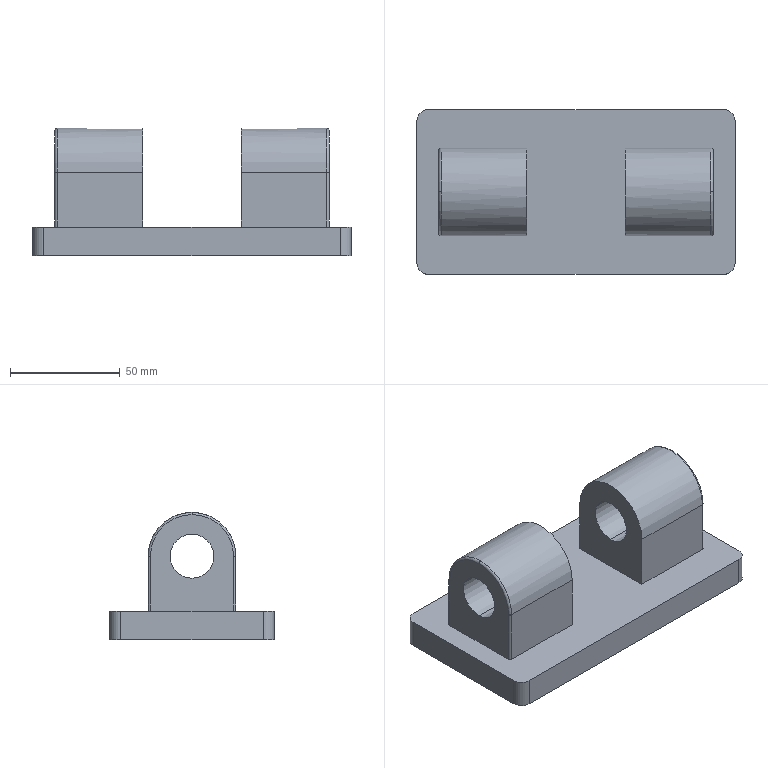Part | STEP file | Hinge lug widened | 1 solid | 32 faces | box 145 x 75 x 58 mm | volume 246181 mm3 | cylinder 14 | plane 14 | torus 4 | commonest cylinder face diameters 2 x4 10 x4 20 x4 40 x2
STEP:
#1=CARTESIAN_POINT('',(57.873,-48.431,650.5));
#2=VERTEX_POINT('',#1);
#3=CARTESIAN_POINT('',(57.873,-48.431,670.5));
#4=VERTEX_POINT('',#3);
#5=CARTESIAN_POINT('',(57.873,-48.431,660.5));
#6=DIRECTION('',(-1.,0.,0.));
#7=DIRECTION('',(0.,0.,1.));
#8=AXIS2_PLACEMENT_3D('',#5,#6,#7);
#9=CIRCLE('',#8,10.);
#10=EDGE_CURVE('',#2,#4,#9,.T.);
#11=ORIENTED_EDGE('',*,*,#10,.F.);
#12=CARTESIAN_POINT('',(17.873,-48.431,650.5));
#13=VERTEX_POINT('',#12);
#14=CARTESIAN_POINT('',(67.873,-48.431,650.5));
#15=DIRECTION('',(-1.,0.,0.));
#16=VECTOR('',#15,1000.);
#17=LINE('',#14,#16);
#18=EDGE_CURVE('',#2,#13,#17,.T.);
#19=ORIENTED_EDGE('',*,*,#18,.T.);
#20=CARTESIAN_POINT('',(17.873,-48.431,670.5));
#21=VERTEX_POINT('',#20);
#22=CARTESIAN_POINT('',(17.873,-48.431,660.5));
#23=DIRECTION('',(-1.,0.,0.));
#24=DIRECTION('',(0.,0.,-1.));
#25=AXIS2_PLACEMENT_3D('',#22,#23,#24);
#26=CIRCLE('',#25,10.);
#27=EDGE_CURVE('',#13,#21,#26,.T.);
#28=ORIENTED_EDGE('',*,*,#27,.T.);
#29=CARTESIAN_POINT('',(67.873,-48.431,670.5));
#30=DIRECTION('',(-1.,0.,0.));
#31=VECTOR('',#30,1000.);
#32=LINE('',#29,#31);
#33=EDGE_CURVE('',#4,#21,#32,.T.);
#34=ORIENTED_EDGE('',*,*,#33,.F.);
#35=EDGE_LOOP('',(#11,#19,#28,#34));
#36=FACE_OUTER_BOUND('',#35,.T.);
#37=CARTESIAN_POINT('',(67.873,-48.431,660.5));
#38=DIRECTION('',(-1.,0.,0.));
#39=DIRECTION('',(0.,0.,1.));
#40=AXIS2_PLACEMENT_3D('',#37,#38,#39);
#41=CYLINDRICAL_SURFACE('',#40,10.);
#42=ADVANCED_FACE('',(#36),#41,.F.);
#43=CARTESIAN_POINT('',(-27.127,-48.431,650.5));
#44=VERTEX_POINT('',#43);
#45=CARTESIAN_POINT('',(-27.127,-48.431,670.5));
#46=VERTEX_POINT('',#45);
#47=CARTESIAN_POINT('',(-27.127,-48.431,660.5));
#48=DIRECTION('',(-1.,0.,0.));
#49=DIRECTION('',(0.,0.,-1.));
#50=AXIS2_PLACEMENT_3D('',#47,#48,#49);
#51=CIRCLE('',#50,10.);
#52=EDGE_CURVE('',#44,#46,#51,.T.);
#53=ORIENTED_EDGE('',*,*,#52,.F.);
#54=CARTESIAN_POINT('',(-67.127,-48.431,650.5));
#55=VERTEX_POINT('',#54);
#56=CARTESIAN_POINT('',(7.873,-48.431,650.5));
#57=DIRECTION('',(-1.,0.,0.));
#58=VECTOR('',#57,1000.);
#59=LINE('',#56,#58);
#60=EDGE_CURVE('',#44,#55,#59,.T.);
#61=ORIENTED_EDGE('',*,*,#60,.T.);
#62=CARTESIAN_POINT('',(-67.127,-48.431,670.5));
#63=VERTEX_POINT('',#62);
#64=CARTESIAN_POINT('',(-67.127,-48.431,660.5));
#65=DIRECTION('',(-1.,0.,0.));
#66=DIRECTION('',(0.,0.,1.));
#67=AXIS2_PLACEMENT_3D('',#64,#65,#66);
#68=CIRCLE('',#67,10.);
#69=EDGE_CURVE('',#55,#63,#68,.T.);
#70=ORIENTED_EDGE('',*,*,#69,.T.);
#71=CARTESIAN_POINT('',(7.873,-48.431,670.5));
#72=DIRECTION('',(-1.,0.,0.));
#73=VECTOR('',#72,1000.);
#74=LINE('',#71,#73);
#75=EDGE_CURVE('',#46,#63,#74,.T.);
#76=ORIENTED_EDGE('',*,*,#75,.F.);
#77=EDGE_LOOP('',(#53,#61,#70,#76));
#78=FACE_OUTER_BOUND('',#77,.T.);
#79=CARTESIAN_POINT('',(7.873,-48.431,660.5));
#80=DIRECTION('',(-1.,0.,0.));
#81=DIRECTION('',(0.,0.,1.));
#82=AXIS2_PLACEMENT_3D('',#79,#80,#81);
#83=CYLINDRICAL_SURFACE('',#82,10.);
#84=ADVANCED_FACE('',(#78),#83,.F.);
#85=CARTESIAN_POINT('',(17.873,-28.431,635.5));
#86=VERTEX_POINT('',#85);
#87=CARTESIAN_POINT('',(17.873,-68.431,635.5));
#88=VERTEX_POINT('',#87);
#89=CARTESIAN_POINT('',(17.873,-58.431,635.5));
#90=DIRECTION('',(0.,-1.,0.));
#91=VECTOR('',#90,1000.);
#92=LINE('',#89,#91);
#93=EDGE_CURVE('',#86,#88,#92,.T.);
#94=ORIENTED_EDGE('',*,*,#93,.F.);
#95=CARTESIAN_POINT('',(56.873,-28.431,635.5));
#96=VERTEX_POINT('',#95);
#97=CARTESIAN_POINT('',(57.873,-28.431,635.5));
#98=DIRECTION('',(-1.,0.,0.));
#99=VECTOR('',#98,1000.);
#100=LINE('',#97,#99);
#101=EDGE_CURVE('',#96,#86,#100,.T.);
#102=ORIENTED_EDGE('',*,*,#101,.F.);
#103=CARTESIAN_POINT('',(57.873,-29.431,635.5));
#104=VERTEX_POINT('',#103);
#105=CARTESIAN_POINT('',(56.873,-29.431,635.5));
#106=DIRECTION('',(0.,0.,-1.));
#107=DIRECTION('',(1.,0.,0.));
#108=AXIS2_PLACEMENT_3D('',#105,#106,#107);
#109=CIRCLE('',#108,1.);
#110=EDGE_CURVE('',#96,#104,#109,.T.);
#111=ORIENTED_EDGE('',*,*,#110,.T.);
#112=CARTESIAN_POINT('',(57.873,-67.431,635.5));
#113=VERTEX_POINT('',#112);
#114=CARTESIAN_POINT('',(57.873,-28.431,635.5));
#115=DIRECTION('',(0.,1.,0.));
#116=VECTOR('',#115,1000.);
#117=LINE('',#114,#116);
#118=EDGE_CURVE('',#113,#104,#117,.T.);
#119=ORIENTED_EDGE('',*,*,#118,.F.);
#120=CARTESIAN_POINT('',(56.873,-68.431,635.5));
#121=VERTEX_POINT('',#120);
#122=CARTESIAN_POINT('',(56.873,-67.431,635.5));
#123=DIRECTION('',(0.,0.,-1.));
#124=DIRECTION('',(1.,0.,0.));
#125=AXIS2_PLACEMENT_3D('',#122,#123,#124);
#126=CIRCLE('',#125,1.);
#127=EDGE_CURVE('',#113,#121,#126,.T.);
#128=ORIENTED_EDGE('',*,*,#127,.T.);
#129=CARTESIAN_POINT('',(57.873,-68.431,635.5));
#130=DIRECTION('',(1.,0.,0.));
#131=VECTOR('',#130,1000.);
#132=LINE('',#129,#131);
#133=EDGE_CURVE('',#88,#121,#132,.T.);
#134=ORIENTED_EDGE('',*,*,#133,.F.);
#135=EDGE_LOOP('',(#94,#102,#111,#119,#128,#134));
#136=FACE_BOUND('',#135,.T.);
#137=CARTESIAN_POINT('',(62.873,-85.931,635.5));
#138=VERTEX_POINT('',#137);
#139=CARTESIAN_POINT('',(-72.127,-85.931,635.5));
#140=VERTEX_POINT('',#139);
#141=CARTESIAN_POINT('',(-77.127,-85.931,635.5));
#142=DIRECTION('',(-1.,0.,0.));
#143=VECTOR('',#142,1000.);
#144=LINE('',#141,#143);
#145=EDGE_CURVE('',#138,#140,#144,.T.);
#146=ORIENTED_EDGE('',*,*,#145,.F.);
#147=CARTESIAN_POINT('',(67.873,-80.931,635.5));
#148=VERTEX_POINT('',#147);
#149=CARTESIAN_POINT('',(62.873,-80.931,635.5));
#150=DIRECTION('',(0.,0.,1.));
#151=DIRECTION('',(1.,0.,0.));
#152=AXIS2_PLACEMENT_3D('',#149,#150,#151);
#153=CIRCLE('',#152,5.);
#154=EDGE_CURVE('',#138,#148,#153,.T.);
#155=ORIENTED_EDGE('',*,*,#154,.T.);
#156=CARTESIAN_POINT('',(67.873,-15.931,635.5));
#157=VERTEX_POINT('',#156);
#158=CARTESIAN_POINT('',(67.873,-10.931,635.5));
#159=DIRECTION('',(0.,-1.,0.));
#160=VECTOR('',#159,1000.);
#161=LINE('',#158,#160);
#162=EDGE_CURVE('',#157,#148,#161,.T.);
#163=ORIENTED_EDGE('',*,*,#162,.F.);
#164=CARTESIAN_POINT('',(62.873,-10.931,635.5));
#165=VERTEX_POINT('',#164);
#166=CARTESIAN_POINT('',(62.873,-15.931,635.5));
#167=DIRECTION('',(0.,0.,1.));
#168=DIRECTION('',(1.,0.,0.));
#169=AXIS2_PLACEMENT_3D('',#166,#167,#168);
#170=CIRCLE('',#169,5.);
#171=EDGE_CURVE('',#157,#165,#170,.T.);
#172=ORIENTED_EDGE('',*,*,#171,.T.);
#173=CARTESIAN_POINT('',(-72.127,-10.931,635.5));
#174=VERTEX_POINT('',#173);
#175=CARTESIAN_POINT('',(-77.127,-10.931,635.5));
#176=DIRECTION('',(1.,0.,0.));
#177=VECTOR('',#176,1000.);
#178=LINE('',#175,#177);
#179=EDGE_CURVE('',#174,#165,#178,.T.);
#180=ORIENTED_EDGE('',*,*,#179,.F.);
#181=CARTESIAN_POINT('',(-77.127,-15.931,635.5));
#182=VERTEX_POINT('',#181);
#183=CARTESIAN_POINT('',(-72.127,-15.931,635.5));
#184=DIRECTION('',(0.,0.,1.));
#185=DIRECTION('',(1.,0.,0.));
#186=AXIS2_PLACEMENT_3D('',#183,#184,#185);
#187=CIRCLE('',#186,5.);
#188=EDGE_CURVE('',#174,#182,#187,.T.);
#189=ORIENTED_EDGE('',*,*,#188,.T.);
#190=CARTESIAN_POINT('',(-77.127,-80.931,635.5));
#191=VERTEX_POINT('',#190);
#192=CARTESIAN_POINT('',(-77.127,-10.931,635.5));
#193=DIRECTION('',(0.,1.,0.));
#194=VECTOR('',#193,1000.);
#195=LINE('',#192,#194);
#196=EDGE_CURVE('',#191,#182,#195,.T.);
#197=ORIENTED_EDGE('',*,*,#196,.F.);
#198=CARTESIAN_POINT('',(-72.127,-80.931,635.5));
#199=DIRECTION('',(0.,0.,1.));
#200=DIRECTION('',(1.,0.,0.));
#201=AXIS2_PLACEMENT_3D('',#198,#199,#200);
#202=CIRCLE('',#201,5.);
#203=EDGE_CURVE('',#191,#140,#202,.T.);
#204=ORIENTED_EDGE('',*,*,#203,.T.);
#205=EDGE_LOOP('',(#146,#155,#163,#172,#180,#189,#197,#204));
#206=FACE_OUTER_BOUND('',#205,.T.);
#207=CARTESIAN_POINT('',(-27.127,-28.431,635.5));
#208=VERTEX_POINT('',#207);
#209=CARTESIAN_POINT('',(-66.127,-28.431,635.5));
#210=VERTEX_POINT('',#209);
#211=CARTESIAN_POINT('',(-67.127,-28.431,635.5));
#212=DIRECTION('',(-1.,0.,0.));
#213=VECTOR('',#212,1000.);
#214=LINE('',#211,#213);
#215=EDGE_CURVE('',#208,#210,#214,.T.);
#216=ORIENTED_EDGE('',*,*,#215,.F.);
#217=CARTESIAN_POINT('',(-27.127,-68.431,635.5));
#218=VERTEX_POINT('',#217);
#219=CARTESIAN_POINT('',(-27.127,-58.431,635.5));
#220=DIRECTION('',(0.,-1.,0.));
#221=VECTOR('',#220,1000.);
#222=LINE('',#219,#221);
#223=EDGE_CURVE('',#208,#218,#222,.T.);
#224=ORIENTED_EDGE('',*,*,#223,.T.);
#225=CARTESIAN_POINT('',(-66.127,-68.431,635.5));
#226=VERTEX_POINT('',#225);
#227=CARTESIAN_POINT('',(-67.127,-68.431,635.5));
#228=DIRECTION('',(1.,0.,0.));
#229=VECTOR('',#228,1000.);
#230=LINE('',#227,#229);
#231=EDGE_CURVE('',#226,#218,#230,.T.);
#232=ORIENTED_EDGE('',*,*,#231,.F.);
#233=CARTESIAN_POINT('',(-67.127,-67.431,635.5));
#234=VERTEX_POINT('',#233);
#235=CARTESIAN_POINT('',(-66.127,-67.431,635.5));
#236=DIRECTION('',(0.,0.,-1.));
#237=DIRECTION('',(1.,0.,0.));
#238=AXIS2_PLACEMENT_3D('',#235,#236,#237);
#239=CIRCLE('',#238,1.);
#240=EDGE_CURVE('',#226,#234,#239,.T.);
#241=ORIENTED_EDGE('',*,*,#240,.T.);
#242=CARTESIAN_POINT('',(-67.127,-29.431,635.5));
#243=VERTEX_POINT('',#242);
#244=CARTESIAN_POINT('',(-67.127,-28.431,635.5));
#245=DIRECTION('',(0.,-1.,0.));
#246=VECTOR('',#245,1000.);
#247=LINE('',#244,#246);
#248=EDGE_CURVE('',#243,#234,#247,.T.);
#249=ORIENTED_EDGE('',*,*,#248,.F.);
#250=CARTESIAN_POINT('',(-66.127,-29.431,635.5));
#251=DIRECTION('',(0.,0.,-1.));
#252=DIRECTION('',(1.,0.,0.));
#253=AXIS2_PLACEMENT_3D('',#250,#251,#252);
#254=CIRCLE('',#253,1.);
#255=EDGE_CURVE('',#243,#210,#254,.T.);
#256=ORIENTED_EDGE('',*,*,#255,.T.);
#257=EDGE_LOOP('',(#216,#224,#232,#241,#249,#256));
#258=FACE_BOUND('',#257,.T.);
#259=CARTESIAN_POINT('',(-34.627,-48.431,635.5));
#260=DIRECTION('',(0.,0.,1.));
#261=DIRECTION('',(0.,-1.,0.));
#262=AXIS2_PLACEMENT_3D('',#259,#260,#261);
#263=PLANE('',#262);
#264=ADVANCED_FACE('',(#136,#206,#258),#263,.T.);
#265=ORIENTED_EDGE('',*,*,#179,.T.);
#266=CARTESIAN_POINT('',(62.873,-10.931,622.5));
#267=VERTEX_POINT('',#266);
#268=CARTESIAN_POINT('',(62.873,-10.931,622.5));
#269=DIRECTION('',(0.,0.,-1.));
#270=VECTOR('',#269,1000.);
#271=LINE('',#268,#270);
#272=EDGE_CURVE('',#165,#267,#271,.T.);
#273=ORIENTED_EDGE('',*,*,#272,.T.);
#274=CARTESIAN_POINT('',(-72.127,-10.931,622.5));
#275=VERTEX_POINT('',#274);
#276=CARTESIAN_POINT('',(-77.127,-10.931,622.5));
#277=DIRECTION('',(1.,0.,0.));
#278=VECTOR('',#277,1000.);
#279=LINE('',#276,#278);
#280=EDGE_CURVE('',#275,#267,#279,.T.);
#281=ORIENTED_EDGE('',*,*,#280,.F.);
#282=CARTESIAN_POINT('',(-72.127,-10.931,622.5));
#283=DIRECTION('',(0.,0.,1.));
#284=VECTOR('',#283,1000.);
#285=LINE('',#282,#284);
#286=EDGE_CURVE('',#275,#174,#285,.T.);
#287=ORIENTED_EDGE('',*,*,#286,.T.);
#288=EDGE_LOOP('',(#265,#273,#281,#287));
#289=FACE_OUTER_BOUND('',#288,.T.);
#290=CARTESIAN_POINT('',(-77.127,-10.931,622.5));
#291=DIRECTION('',(0.,-1.,0.));
#292=DIRECTION('',(0.,0.,1.));
#293=AXIS2_PLACEMENT_3D('',#290,#291,#292);
#294=PLANE('',#293);
#295=ADVANCED_FACE('',(#289),#294,.F.);
#296=CARTESIAN_POINT('',(62.873,-85.931,622.5));
#297=VERTEX_POINT('',#296);
#298=CARTESIAN_POINT('',(-72.127,-85.931,622.5));
#299=VERTEX_POINT('',#298);
#300=CARTESIAN_POINT('',(-77.127,-85.931,622.5));
#301=DIRECTION('',(-1.,0.,0.));
#302=VECTOR('',#301,1000.);
#303=LINE('',#300,#302);
#304=EDGE_CURVE('',#297,#299,#303,.T.);
#305=ORIENTED_EDGE('',*,*,#304,.F.);
#306=CARTESIAN_POINT('',(62.873,-85.931,622.5));
#307=DIRECTION('',(0.,0.,1.));
#308=VECTOR('',#307,1000.);
#309=LINE('',#306,#308);
#310=EDGE_CURVE('',#297,#138,#309,.T.);
#311=ORIENTED_EDGE('',*,*,#310,.T.);
#312=ORIENTED_EDGE('',*,*,#145,.T.);
#313=CARTESIAN_POINT('',(-72.127,-85.931,622.5));
#314=DIRECTION('',(0.,0.,-1.));
#315=VECTOR('',#314,1000.);
#316=LINE('',#313,#315);
#317=EDGE_CURVE('',#140,#299,#316,.T.);
#318=ORIENTED_EDGE('',*,*,#317,.T.);
#319=EDGE_LOOP('',(#305,#311,#312,#318));
#320=FACE_OUTER_BOUND('',#319,.T.);
#321=CARTESIAN_POINT('',(-77.127,-85.931,622.5));
#322=DIRECTION('',(0.,1.,0.));
#323=DIRECTION('',(-1.,0.,0.));
#324=AXIS2_PLACEMENT_3D('',#321,#322,#323);
#325=PLANE('',#324);
#326=ADVANCED_FACE('',(#320),#325,.F.);
#327=ORIENTED_EDGE('',*,*,#280,.T.);
#328=CARTESIAN_POINT('',(67.873,-15.931,622.5));
#329=VERTEX_POINT('',#328);
#330=CARTESIAN_POINT('',(62.873,-15.931,622.5));
#331=DIRECTION('',(0.,0.,-1.));
#332=DIRECTION('',(1.,0.,0.));
#333=AXIS2_PLACEMENT_3D('',#330,#331,#332);
#334=CIRCLE('',#333,5.);
#335=EDGE_CURVE('',#267,#329,#334,.T.);
#336=ORIENTED_EDGE('',*,*,#335,.T.);
#337=CARTESIAN_POINT('',(67.873,-80.931,622.5));
#338=VERTEX_POINT('',#337);
#339=CARTESIAN_POINT('',(67.873,-10.931,622.5));
#340=DIRECTION('',(0.,-1.,0.));
#341=VECTOR('',#340,1000.);
#342=LINE('',#339,#341);
#343=EDGE_CURVE('',#329,#338,#342,.T.);
#344=ORIENTED_EDGE('',*,*,#343,.T.);
#345=CARTESIAN_POINT('',(62.873,-80.931,622.5));
#346=DIRECTION('',(0.,0.,-1.));
#347=DIRECTION('',(1.,0.,0.));
#348=AXIS2_PLACEMENT_3D('',#345,#346,#347);
#349=CIRCLE('',#348,5.);
#350=EDGE_CURVE('',#338,#297,#349,.T.);
#351=ORIENTED_EDGE('',*,*,#350,.T.);
#352=ORIENTED_EDGE('',*,*,#304,.T.);
#353=CARTESIAN_POINT('',(-77.127,-80.931,622.5));
#354=VERTEX_POINT('',#353);
#355=CARTESIAN_POINT('',(-72.127,-80.931,622.5));
#356=DIRECTION('',(0.,0.,-1.));
#357=DIRECTION('',(1.,0.,0.));
#358=AXIS2_PLACEMENT_3D('',#355,#356,#357);
#359=CIRCLE('',#358,5.);
#360=EDGE_CURVE('',#299,#354,#359,.T.);
#361=ORIENTED_EDGE('',*,*,#360,.T.);
#362=CARTESIAN_POINT('',(-77.127,-15.931,622.5));
#363=VERTEX_POINT('',#362);
#364=CARTESIAN_POINT('',(-77.127,-10.931,622.5));
#365=DIRECTION('',(0.,1.,0.));
#366=VECTOR('',#365,1000.);
#367=LINE('',#364,#366);
#368=EDGE_CURVE('',#354,#363,#367,.T.);
#369=ORIENTED_EDGE('',*,*,#368,.T.);
#370=CARTESIAN_POINT('',(-72.127,-15.931,622.5));
#371=DIRECTION('',(0.,0.,-1.));
#372=DIRECTION('',(1.,0.,0.));
#373=AXIS2_PLACEMENT_3D('',#370,#371,#372);
#374=CIRCLE('',#373,5.);
#375=EDGE_CURVE('',#363,#275,#374,.T.);
#376=ORIENTED_EDGE('',*,*,#375,.T.);
#377=EDGE_LOOP('',(#327,#336,#344,#351,#352,#361,#369,#376));
#378=FACE_OUTER_BOUND('',#377,.T.);
#379=CARTESIAN_POINT('',(-34.627,-48.431,622.5));
#380=DIRECTION('',(0.,0.,1.));
#381=DIRECTION('',(0.,-1.,0.));
#382=AXIS2_PLACEMENT_3D('',#379,#380,#381);
#383=PLANE('',#382);
#384=ADVANCED_FACE('',(#378),#383,.F.);
#385=ORIENTED_EDGE('',*,*,#60,.F.);
#386=CARTESIAN_POINT('',(-27.127,-48.431,660.5));
#387=DIRECTION('',(-1.,0.,0.));
#388=DIRECTION('',(0.,0.,-1.));
#389=AXIS2_PLACEMENT_3D('',#386,#387,#388);
#390=CIRCLE('',#389,10.);
#391=EDGE_CURVE('',#46,#44,#390,.T.);
#392=ORIENTED_EDGE('',*,*,#391,.F.);
#393=ORIENTED_EDGE('',*,*,#75,.T.);
#394=CARTESIAN_POINT('',(-67.127,-48.431,660.5));
#395=DIRECTION('',(-1.,0.,0.));
#396=DIRECTION('',(0.,0.,1.));
#397=AXIS2_PLACEMENT_3D('',#394,#395,#396);
#398=CIRCLE('',#397,10.);
#399=EDGE_CURVE('',#63,#55,#398,.T.);
#400=ORIENTED_EDGE('',*,*,#399,.T.);
#401=EDGE_LOOP('',(#385,#392,#393,#400));
#402=FACE_OUTER_BOUND('',#401,.T.);
#403=CARTESIAN_POINT('',(7.873,-48.431,660.5));
#404=DIRECTION('',(-1.,0.,0.));
#405=DIRECTION('',(0.,0.,1.));
#406=AXIS2_PLACEMENT_3D('',#403,#404,#405);
#407=CYLINDRICAL_SURFACE('',#406,10.);
#408=ADVANCED_FACE('',(#402),#407,.F.);
#409=ORIENTED_EDGE('',*,*,#196,.T.);
#410=CARTESIAN_POINT('',(-77.127,-15.931,622.5));
#411=DIRECTION('',(0.,0.,-1.));
#412=VECTOR('',#411,1000.);
#413=LINE('',#410,#412);
#414=EDGE_CURVE('',#182,#363,#413,.T.);
#415=ORIENTED_EDGE('',*,*,#414,.T.);
#416=ORIENTED_EDGE('',*,*,#368,.F.);
#417=CARTESIAN_POINT('',(-77.127,-80.931,622.5));
#418=DIRECTION('',(0.,0.,1.));
#419=VECTOR('',#418,1000.);
#420=LINE('',#417,#419);
#421=EDGE_CURVE('',#354,#191,#420,.T.);
#422=ORIENTED_EDGE('',*,*,#421,.T.);
#423=EDGE_LOOP('',(#409,#415,#416,#422));
#424=FACE_OUTER_BOUND('',#423,.T.);
#425=CARTESIAN_POINT('',(-77.127,-10.931,622.5));
#426=DIRECTION('',(1.,0.,0.));
#427=DIRECTION('',(0.,1.,0.));
#428=AXIS2_PLACEMENT_3D('',#425,#426,#427);
#429=PLANE('',#428);
#430=ADVANCED_FACE('',(#424),#429,.F.);
#431=ORIENTED_EDGE('',*,*,#248,.T.);
#432=CARTESIAN_POINT('',(-67.127,-67.431,660.5));
#433=VERTEX_POINT('',#432);
#434=CARTESIAN_POINT('',(-67.127,-67.431,680.5));
#435=DIRECTION('',(0.,0.,1.));
#436=VECTOR('',#435,1000.);
#437=LINE('',#434,#436);
#438=EDGE_CURVE('',#234,#433,#437,.T.);
#439=ORIENTED_EDGE('',*,*,#438,.T.);
#440=CARTESIAN_POINT('',(-67.127,-48.431,679.5));
#441=VERTEX_POINT('',#440);
#442=CARTESIAN_POINT('',(-67.127,-48.431,660.5));
#443=DIRECTION('',(-1.,0.,0.));
#444=DIRECTION('',(0.,0.,-1.));
#445=AXIS2_PLACEMENT_3D('',#442,#443,#444);
#446=CIRCLE('',#445,19.);
#447=EDGE_CURVE('',#433,#441,#446,.T.);
#448=ORIENTED_EDGE('',*,*,#447,.T.);
#449=CARTESIAN_POINT('',(-67.127,-29.431,660.5));
#450=VERTEX_POINT('',#449);
#451=CARTESIAN_POINT('',(-67.127,-48.431,660.5));
#452=DIRECTION('',(-1.,0.,0.));
#453=DIRECTION('',(0.,0.,-1.));
#454=AXIS2_PLACEMENT_3D('',#451,#452,#453);
#455=CIRCLE('',#454,19.);
#456=EDGE_CURVE('',#441,#450,#455,.T.);
#457=ORIENTED_EDGE('',*,*,#456,.T.);
#458=CARTESIAN_POINT('',(-67.127,-29.431,680.5));
#459=DIRECTION('',(0.,0.,-1.));
#460=VECTOR('',#459,1000.);
#461=LINE('',#458,#460);
#462=EDGE_CURVE('',#450,#243,#461,.T.);
#463=ORIENTED_EDGE('',*,*,#462,.T.);
#464=EDGE_LOOP('',(#431,#439,#448,#457,#463));
#465=FACE_OUTER_BOUND('',#464,.T.);
#466=ORIENTED_EDGE('',*,*,#399,.F.);
#467=ORIENTED_EDGE('',*,*,#69,.F.);
#468=EDGE_LOOP('',(#466,#467));
#469=FACE_BOUND('',#468,.T.);
#470=CARTESIAN_POINT('',(-67.127,-28.431,680.5));
#471=DIRECTION('',(1.,0.,0.));
#472=DIRECTION('',(0.,0.,-1.));
#473=AXIS2_PLACEMENT_3D('',#470,#471,#472);
#474=PLANE('',#473);
#475=ADVANCED_FACE('',(#465,#469),#474,.F.);
#476=ORIENTED_EDGE('',*,*,#231,.T.);
#477=CARTESIAN_POINT('',(-27.127,-68.431,660.5));
#478=VERTEX_POINT('',#477);
#479=CARTESIAN_POINT('',(-27.127,-68.431,635.5));
#480=DIRECTION('',(0.,0.,1.));
#481=VECTOR('',#480,1000.);
#482=LINE('',#479,#481);
#483=EDGE_CURVE('',#218,#478,#482,.T.);
#484=ORIENTED_EDGE('',*,*,#483,.T.);
#485=CARTESIAN_POINT('',(-66.127,-68.431,660.5));
#486=VERTEX_POINT('',#485);
#487=CARTESIAN_POINT('',(-67.127,-68.431,660.5));
#488=DIRECTION('',(-1.,0.,0.));
#489=VECTOR('',#488,1000.);
#490=LINE('',#487,#489);
#491=EDGE_CURVE('',#478,#486,#490,.T.);
#492=ORIENTED_EDGE('',*,*,#491,.T.);
#493=CARTESIAN_POINT('',(-66.127,-68.431,680.5));
#494=DIRECTION('',(0.,0.,-1.));
#495=VECTOR('',#494,1000.);
#496=LINE('',#493,#495);
#497=EDGE_CURVE('',#486,#226,#496,.T.);
#498=ORIENTED_EDGE('',*,*,#497,.T.);
#499=EDGE_LOOP('',(#476,#484,#492,#498));
#500=FACE_OUTER_BOUND('',#499,.T.);
#501=CARTESIAN_POINT('',(-67.127,-68.431,680.5));
#502=DIRECTION('',(0.,1.,0.));
#503=DIRECTION('',(-1.,0.,0.));
#504=AXIS2_PLACEMENT_3D('',#501,#502,#503);
#505=PLANE('',#504);
#506=ADVANCED_FACE('',(#500),#505,.F.);
#507=CARTESIAN_POINT('',(-66.127,-28.431,660.5));
#508=VERTEX_POINT('',#507);
#509=CARTESIAN_POINT('',(-27.127,-28.431,660.5));
#510=VERTEX_POINT('',#509);
#511=CARTESIAN_POINT('',(-47.127,-28.431,660.5));
#512=DIRECTION('',(1.,0.,0.));
#513=VECTOR('',#512,1000.);
#514=LINE('',#511,#513);
#515=EDGE_CURVE('',#508,#510,#514,.T.);
#516=ORIENTED_EDGE('',*,*,#515,.T.);
#517=CARTESIAN_POINT('',(-27.127,-28.431,660.5));
#518=DIRECTION('',(0.,0.,-1.));
#519=VECTOR('',#518,1000.);
#520=LINE('',#517,#519);
#521=EDGE_CURVE('',#510,#208,#520,.T.);
#522=ORIENTED_EDGE('',*,*,#521,.T.);
#523=ORIENTED_EDGE('',*,*,#215,.T.);
#524=CARTESIAN_POINT('',(-66.127,-28.431,680.5));
#525=DIRECTION('',(0.,0.,1.));
#526=VECTOR('',#525,1000.);
#527=LINE('',#524,#526);
#528=EDGE_CURVE('',#210,#508,#527,.T.);
#529=ORIENTED_EDGE('',*,*,#528,.T.);
#530=EDGE_LOOP('',(#516,#522,#523,#529));
#531=FACE_OUTER_BOUND('',#530,.T.);
#532=CARTESIAN_POINT('',(-67.127,-28.431,680.5));
#533=DIRECTION('',(0.,-1.,0.));
#534=DIRECTION('',(0.,0.,1.));
#535=AXIS2_PLACEMENT_3D('',#532,#533,#534);
#536=PLANE('',#535);
#537=ADVANCED_FACE('',(#531),#536,.F.);
#538=CARTESIAN_POINT('',(-66.127,-48.431,680.5));
#539=VERTEX_POINT('',#538);
#540=CARTESIAN_POINT('',(-66.127,-48.431,660.5));
#541=DIRECTION('',(1.,0.,0.));
#542=DIRECTION('',(0.,0.,-1.));
#543=AXIS2_PLACEMENT_3D('',#540,#541,#542);
#544=CIRCLE('',#543,20.);
#545=EDGE_CURVE('',#508,#539,#544,.T.);
#546=ORIENTED_EDGE('',*,*,#545,.T.);
#547=CARTESIAN_POINT('',(-66.127,-48.431,660.5));
#548=DIRECTION('',(1.,0.,0.));
#549=DIRECTION('',(0.,0.,-1.));
#550=AXIS2_PLACEMENT_3D('',#547,#548,#549);
#551=CIRCLE('',#550,20.);
#552=EDGE_CURVE('',#539,#486,#551,.T.);
#553=ORIENTED_EDGE('',*,*,#552,.T.);
#554=ORIENTED_EDGE('',*,*,#491,.F.);
#555=CARTESIAN_POINT('',(-27.127,-48.431,660.5));
#556=DIRECTION('',(-1.,0.,0.));
#557=DIRECTION('',(0.,0.,-1.));
#558=AXIS2_PLACEMENT_3D('',#555,#556,#557);
#559=CIRCLE('',#558,20.);
#560=EDGE_CURVE('',#478,#510,#559,.T.);
#561=ORIENTED_EDGE('',*,*,#560,.T.);
#562=ORIENTED_EDGE('',*,*,#515,.F.);
#563=EDGE_LOOP('',(#546,#553,#554,#561,#562));
#564=FACE_OUTER_BOUND('',#563,.T.);
#565=CARTESIAN_POINT('',(-34.627,-48.431,660.5));
#566=DIRECTION('',(1.,0.,0.));
#567=DIRECTION('',(0.,0.,-1.));
#568=AXIS2_PLACEMENT_3D('',#565,#566,#567);
#569=CYLINDRICAL_SURFACE('',#568,20.);
#570=ADVANCED_FACE('',(#564),#569,.T.);
#571=ORIENTED_EDGE('',*,*,#255,.F.);
#572=ORIENTED_EDGE('',*,*,#462,.F.);
#573=CARTESIAN_POINT('',(-66.127,-29.431,660.5));
#574=DIRECTION('',(0.,0.,1.));
#575=DIRECTION('',(1.,0.,0.));
#576=AXIS2_PLACEMENT_3D('',#573,#574,#575);
#577=CIRCLE('',#576,1.);
#578=EDGE_CURVE('',#508,#450,#577,.T.);
#579=ORIENTED_EDGE('',*,*,#578,.F.);
#580=ORIENTED_EDGE('',*,*,#528,.F.);
#581=EDGE_LOOP('',(#571,#572,#579,#580));
#582=FACE_OUTER_BOUND('',#581,.T.);
#583=CARTESIAN_POINT('',(-66.127,-29.431,680.5));
#584=DIRECTION('',(0.,0.,-1.));
#585=DIRECTION('',(-1.,0.,0.));
#586=AXIS2_PLACEMENT_3D('',#583,#584,#585);
#587=CYLINDRICAL_SURFACE('',#586,1.);
#588=ADVANCED_FACE('',(#582),#587,.T.);
#589=ORIENTED_EDGE('',*,*,#578,.T.);
#590=ORIENTED_EDGE('',*,*,#456,.F.);
#591=CARTESIAN_POINT('',(-66.127,-48.431,679.5));
#592=DIRECTION('',(0.,-1.,0.));
#593=DIRECTION('',(-1.,0.,0.));
#594=AXIS2_PLACEMENT_3D('',#591,#592,#593);
#595=CIRCLE('',#594,1.);
#596=EDGE_CURVE('',#539,#441,#595,.T.);
#597=ORIENTED_EDGE('',*,*,#596,.F.);
#598=ORIENTED_EDGE('',*,*,#545,.F.);
#599=EDGE_LOOP('',(#589,#590,#597,#598));
#600=FACE_OUTER_BOUND('',#599,.T.);
#601=CARTESIAN_POINT('',(-66.127,-48.431,660.5));
#602=DIRECTION('',(1.,0.,0.));
#603=DIRECTION('',(0.,0.,-1.));
#604=AXIS2_PLACEMENT_3D('',#601,#602,#603);
#605=TOROIDAL_SURFACE('',#604,19.,1.);
#606=ADVANCED_FACE('',(#600),#605,.T.);
#607=ORIENTED_EDGE('',*,*,#596,.T.);
#608=ORIENTED_EDGE('',*,*,#447,.F.);
#609=CARTESIAN_POINT('',(-66.127,-67.431,660.5));
#610=DIRECTION('',(0.,0.,-1.));
#611=DIRECTION('',(-1.,0.,0.));
#612=AXIS2_PLACEMENT_3D('',#609,#610,#611);
#613=CIRCLE('',#612,1.);
#614=EDGE_CURVE('',#486,#433,#613,.T.);
#615=ORIENTED_EDGE('',*,*,#614,.F.);
#616=ORIENTED_EDGE('',*,*,#552,.F.);
#617=EDGE_LOOP('',(#607,#608,#615,#616));
#618=FACE_OUTER_BOUND('',#617,.T.);
#619=CARTESIAN_POINT('',(-66.127,-48.431,660.5));
#620=DIRECTION('',(1.,0.,0.));
#621=DIRECTION('',(0.,0.,-1.));
#622=AXIS2_PLACEMENT_3D('',#619,#620,#621);
#623=TOROIDAL_SURFACE('',#622,19.,1.);
#624=ADVANCED_FACE('',(#618),#623,.T.);
#625=ORIENTED_EDGE('',*,*,#614,.T.);
#626=ORIENTED_EDGE('',*,*,#438,.F.);
#627=ORIENTED_EDGE('',*,*,#240,.F.);
#628=ORIENTED_EDGE('',*,*,#497,.F.);
#629=EDGE_LOOP('',(#625,#626,#627,#628));
#630=FACE_OUTER_BOUND('',#629,.T.);
#631=CARTESIAN_POINT('',(-66.127,-67.431,680.5));
#632=DIRECTION('',(0.,0.,-1.));
#633=DIRECTION('',(-1.,0.,0.));
#634=AXIS2_PLACEMENT_3D('',#631,#632,#633);
#635=CYLINDRICAL_SURFACE('',#634,1.);
#636=ADVANCED_FACE('',(#630),#635,.T.);
#637=ORIENTED_EDGE('',*,*,#375,.F.);
#638=ORIENTED_EDGE('',*,*,#414,.F.);
#639=ORIENTED_EDGE('',*,*,#188,.F.);
#640=ORIENTED_EDGE('',*,*,#286,.F.);
#641=EDGE_LOOP('',(#637,#638,#639,#640));
#642=FACE_OUTER_BOUND('',#641,.T.);
#643=CARTESIAN_POINT('',(-72.127,-15.931,622.5));
#644=DIRECTION('',(0.,0.,1.));
#645=DIRECTION('',(1.,0.,0.));
#646=AXIS2_PLACEMENT_3D('',#643,#644,#645);
#647=CYLINDRICAL_SURFACE('',#646,5.);
#648=ADVANCED_FACE('',(#642),#647,.T.);
#649=ORIENTED_EDGE('',*,*,#360,.F.);
#650=ORIENTED_EDGE('',*,*,#317,.F.);
#651=ORIENTED_EDGE('',*,*,#203,.F.);
#652=ORIENTED_EDGE('',*,*,#421,.F.);
#653=EDGE_LOOP('',(#649,#650,#651,#652));
#654=FACE_OUTER_BOUND('',#653,.T.);
#655=CARTESIAN_POINT('',(-72.127,-80.931,622.5));
#656=DIRECTION('',(0.,0.,1.));
#657=DIRECTION('',(1.,0.,0.));
#658=AXIS2_PLACEMENT_3D('',#655,#656,#657);
#659=CYLINDRICAL_SURFACE('',#658,5.);
#660=ADVANCED_FACE('',(#654),#659,.T.);
#661=CARTESIAN_POINT('',(56.873,-68.431,660.5));
#662=VERTEX_POINT('',#661);
#663=CARTESIAN_POINT('',(17.873,-68.431,660.5));
#664=VERTEX_POINT('',#663);
#665=CARTESIAN_POINT('',(57.873,-68.431,660.5));
#666=DIRECTION('',(-1.,0.,0.));
#667=VECTOR('',#666,1000.);
#668=LINE('',#665,#667);
#669=EDGE_CURVE('',#662,#664,#668,.T.);
#670=ORIENTED_EDGE('',*,*,#669,.F.);
#671=CARTESIAN_POINT('',(56.873,-48.431,680.5));
#672=VERTEX_POINT('',#671);
#673=CARTESIAN_POINT('',(56.873,-48.431,660.5));
#674=DIRECTION('',(-1.,0.,0.));
#675=DIRECTION('',(0.,0.,1.));
#676=AXIS2_PLACEMENT_3D('',#673,#674,#675);
#677=CIRCLE('',#676,20.);
#678=EDGE_CURVE('',#662,#672,#677,.T.);
#679=ORIENTED_EDGE('',*,*,#678,.T.);
#680=CARTESIAN_POINT('',(56.873,-28.431,660.5));
#681=VERTEX_POINT('',#680);
#682=CARTESIAN_POINT('',(56.873,-48.431,660.5));
#683=DIRECTION('',(-1.,0.,0.));
#684=DIRECTION('',(0.,0.,1.));
#685=AXIS2_PLACEMENT_3D('',#682,#683,#684);
#686=CIRCLE('',#685,20.);
#687=EDGE_CURVE('',#672,#681,#686,.T.);
#688=ORIENTED_EDGE('',*,*,#687,.T.);
#689=CARTESIAN_POINT('',(17.873,-28.431,660.5));
#690=VERTEX_POINT('',#689);
#691=CARTESIAN_POINT('',(57.873,-28.431,660.5));
#692=DIRECTION('',(1.,0.,0.));
#693=VECTOR('',#692,1000.);
#694=LINE('',#691,#693);
#695=EDGE_CURVE('',#690,#681,#694,.T.);
#696=ORIENTED_EDGE('',*,*,#695,.F.);
#697=CARTESIAN_POINT('',(17.873,-48.431,660.5));
#698=DIRECTION('',(-1.,0.,0.));
#699=DIRECTION('',(0.,0.,-1.));
#700=AXIS2_PLACEMENT_3D('',#697,#698,#699);
#701=CIRCLE('',#700,20.);
#702=EDGE_CURVE('',#664,#690,#701,.T.);
#703=ORIENTED_EDGE('',*,*,#702,.F.);
#704=EDGE_LOOP('',(#670,#679,#688,#696,#703));
#705=FACE_OUTER_BOUND('',#704,.T.);
#706=CARTESIAN_POINT('',(25.373,-48.431,660.5));
#707=DIRECTION('',(1.,0.,0.));
#708=DIRECTION('',(0.,-1.,0.));
#709=AXIS2_PLACEMENT_3D('',#706,#707,#708);
#710=CYLINDRICAL_SURFACE('',#709,20.);
#711=ADVANCED_FACE('',(#705),#710,.T.);
#712=ORIENTED_EDGE('',*,*,#18,.F.);
#713=CARTESIAN_POINT('',(57.873,-48.431,660.5));
#714=DIRECTION('',(-1.,0.,0.));
#715=DIRECTION('',(0.,0.,1.));
#716=AXIS2_PLACEMENT_3D('',#713,#714,#715);
#717=CIRCLE('',#716,10.);
#718=EDGE_CURVE('',#4,#2,#717,.T.);
#719=ORIENTED_EDGE('',*,*,#718,.F.);
#720=ORIENTED_EDGE('',*,*,#33,.T.);
#721=CARTESIAN_POINT('',(17.873,-48.431,660.5));
#722=DIRECTION('',(-1.,0.,0.));
#723=DIRECTION('',(0.,0.,-1.));
#724=AXIS2_PLACEMENT_3D('',#721,#722,#723);
#725=CIRCLE('',#724,10.);
#726=EDGE_CURVE('',#21,#13,#725,.T.);
#727=ORIENTED_EDGE('',*,*,#726,.T.);
#728=EDGE_LOOP('',(#712,#719,#720,#727));
#729=FACE_OUTER_BOUND('',#728,.T.);
#730=CARTESIAN_POINT('',(67.873,-48.431,660.5));
#731=DIRECTION('',(-1.,0.,0.));
#732=DIRECTION('',(0.,0.,1.));
#733=AXIS2_PLACEMENT_3D('',#730,#731,#732);
#734=CYLINDRICAL_SURFACE('',#733,10.);
#735=ADVANCED_FACE('',(#729),#734,.F.);
#736=CARTESIAN_POINT('',(57.873,-67.431,660.5));
#737=VERTEX_POINT('',#736);
#738=CARTESIAN_POINT('',(56.873,-67.431,660.5));
#739=DIRECTION('',(0.,0.,1.));
#740=DIRECTION('',(1.,0.,0.));
#741=AXIS2_PLACEMENT_3D('',#738,#739,#740);
#742=CIRCLE('',#741,1.);
#743=EDGE_CURVE('',#662,#737,#742,.T.);
#744=ORIENTED_EDGE('',*,*,#743,.T.);
#745=CARTESIAN_POINT('',(57.873,-48.431,679.5));
#746=VERTEX_POINT('',#745);
#747=CARTESIAN_POINT('',(57.873,-48.431,660.5));
#748=DIRECTION('',(1.,0.,0.));
#749=DIRECTION('',(0.,0.,1.));
#750=AXIS2_PLACEMENT_3D('',#747,#748,#749);
#751=CIRCLE('',#750,19.);
#752=EDGE_CURVE('',#746,#737,#751,.T.);
#753=ORIENTED_EDGE('',*,*,#752,.F.);
#754=CARTESIAN_POINT('',(56.873,-48.431,679.5));
#755=DIRECTION('',(0.,1.,0.));
#756=DIRECTION('',(0.,0.,-1.));
#757=AXIS2_PLACEMENT_3D('',#754,#755,#756);
#758=CIRCLE('',#757,1.);
#759=EDGE_CURVE('',#672,#746,#758,.T.);
#760=ORIENTED_EDGE('',*,*,#759,.F.);
#761=ORIENTED_EDGE('',*,*,#678,.F.);
#762=EDGE_LOOP('',(#744,#753,#760,#761));
#763=FACE_OUTER_BOUND('',#762,.T.);
#764=CARTESIAN_POINT('',(56.873,-48.431,660.5));
#765=DIRECTION('',(-1.,0.,0.));
#766=DIRECTION('',(0.,0.,1.));
#767=AXIS2_PLACEMENT_3D('',#764,#765,#766);
#768=TOROIDAL_SURFACE('',#767,19.,1.);
#769=ADVANCED_FACE('',(#763),#768,.T.);
#770=ORIENTED_EDGE('',*,*,#759,.T.);
#771=CARTESIAN_POINT('',(57.873,-29.431,660.5));
#772=VERTEX_POINT('',#771);
#773=CARTESIAN_POINT('',(57.873,-48.431,660.5));
#774=DIRECTION('',(1.,0.,0.));
#775=DIRECTION('',(0.,0.,1.));
#776=AXIS2_PLACEMENT_3D('',#773,#774,#775);
#777=CIRCLE('',#776,19.);
#778=EDGE_CURVE('',#772,#746,#777,.T.);
#779=ORIENTED_EDGE('',*,*,#778,.F.);
#780=CARTESIAN_POINT('',(56.873,-29.431,660.5));
#781=DIRECTION('',(0.,0.,-1.));
#782=DIRECTION('',(-1.,0.,0.));
#783=AXIS2_PLACEMENT_3D('',#780,#781,#782);
#784=CIRCLE('',#783,1.);
#785=EDGE_CURVE('',#681,#772,#784,.T.);
#786=ORIENTED_EDGE('',*,*,#785,.F.);
#787=ORIENTED_EDGE('',*,*,#687,.F.);
#788=EDGE_LOOP('',(#770,#779,#786,#787));
#789=FACE_OUTER_BOUND('',#788,.T.);
#790=CARTESIAN_POINT('',(56.873,-48.431,660.5));
#791=DIRECTION('',(-1.,0.,0.));
#792=DIRECTION('',(0.,0.,1.));
#793=AXIS2_PLACEMENT_3D('',#790,#791,#792);
#794=TOROIDAL_SURFACE('',#793,19.,1.);
#795=ADVANCED_FACE('',(#789),#794,.T.);
#796=ORIENTED_EDGE('',*,*,#133,.T.);
#797=CARTESIAN_POINT('',(56.873,-68.431,680.5));
#798=DIRECTION('',(0.,0.,1.));
#799=VECTOR('',#798,1000.);
#800=LINE('',#797,#799);
#801=EDGE_CURVE('',#121,#662,#800,.T.);
#802=ORIENTED_EDGE('',*,*,#801,.T.);
#803=ORIENTED_EDGE('',*,*,#669,.T.);
#804=CARTESIAN_POINT('',(17.873,-68.431,635.5));
#805=DIRECTION('',(0.,0.,1.));
#806=VECTOR('',#805,1000.);
#807=LINE('',#804,#806);
#808=EDGE_CURVE('',#88,#664,#807,.T.);
#809=ORIENTED_EDGE('',*,*,#808,.F.);
#810=EDGE_LOOP('',(#796,#802,#803,#809));
#811=FACE_OUTER_BOUND('',#810,.T.);
#812=CARTESIAN_POINT('',(57.873,-68.431,680.5));
#813=DIRECTION('',(0.,1.,0.));
#814=DIRECTION('',(-1.,0.,0.));
#815=AXIS2_PLACEMENT_3D('',#812,#813,#814);
#816=PLANE('',#815);
#817=ADVANCED_FACE('',(#811),#816,.F.);
#818=ORIENTED_EDGE('',*,*,#127,.F.);
#819=CARTESIAN_POINT('',(57.873,-67.431,680.5));
#820=DIRECTION('',(0.,0.,-1.));
#821=VECTOR('',#820,1000.);
#822=LINE('',#819,#821);
#823=EDGE_CURVE('',#737,#113,#822,.T.);
#824=ORIENTED_EDGE('',*,*,#823,.F.);
#825=ORIENTED_EDGE('',*,*,#743,.F.);
#826=ORIENTED_EDGE('',*,*,#801,.F.);
#827=EDGE_LOOP('',(#818,#824,#825,#826));
#828=FACE_OUTER_BOUND('',#827,.T.);
#829=CARTESIAN_POINT('',(56.873,-67.431,680.5));
#830=DIRECTION('',(0.,0.,-1.));
#831=DIRECTION('',(-1.,0.,0.));
#832=AXIS2_PLACEMENT_3D('',#829,#830,#831);
#833=CYLINDRICAL_SURFACE('',#832,1.);
#834=ADVANCED_FACE('',(#828),#833,.T.);
#835=ORIENTED_EDGE('',*,*,#118,.T.);
#836=CARTESIAN_POINT('',(57.873,-29.431,680.5));
#837=DIRECTION('',(0.,0.,1.));
#838=VECTOR('',#837,1000.);
#839=LINE('',#836,#838);
#840=EDGE_CURVE('',#104,#772,#839,.T.);
#841=ORIENTED_EDGE('',*,*,#840,.T.);
#842=ORIENTED_EDGE('',*,*,#778,.T.);
#843=ORIENTED_EDGE('',*,*,#752,.T.);
#844=ORIENTED_EDGE('',*,*,#823,.T.);
#845=EDGE_LOOP('',(#835,#841,#842,#843,#844));
#846=FACE_OUTER_BOUND('',#845,.T.);
#847=ORIENTED_EDGE('',*,*,#718,.T.);
#848=ORIENTED_EDGE('',*,*,#10,.T.);
#849=EDGE_LOOP('',(#847,#848));
#850=FACE_BOUND('',#849,.T.);
#851=CARTESIAN_POINT('',(57.873,-28.431,680.5));
#852=DIRECTION('',(-1.,0.,0.));
#853=DIRECTION('',(0.,1.,0.));
#854=AXIS2_PLACEMENT_3D('',#851,#852,#853);
#855=PLANE('',#854);
#856=ADVANCED_FACE('',(#846,#850),#855,.F.);
#857=ORIENTED_EDGE('',*,*,#785,.T.);
#858=ORIENTED_EDGE('',*,*,#840,.F.);
#859=ORIENTED_EDGE('',*,*,#110,.F.);
#860=CARTESIAN_POINT('',(56.873,-28.431,680.5));
#861=DIRECTION('',(0.,0.,-1.));
#862=VECTOR('',#861,1000.);
#863=LINE('',#860,#862);
#864=EDGE_CURVE('',#681,#96,#863,.T.);
#865=ORIENTED_EDGE('',*,*,#864,.F.);
#866=EDGE_LOOP('',(#857,#858,#859,#865));
#867=FACE_OUTER_BOUND('',#866,.T.);
#868=CARTESIAN_POINT('',(56.873,-29.431,680.5));
#869=DIRECTION('',(0.,0.,-1.));
#870=DIRECTION('',(-1.,0.,0.));
#871=AXIS2_PLACEMENT_3D('',#868,#869,#870);
#872=CYLINDRICAL_SURFACE('',#871,1.);
#873=ADVANCED_FACE('',(#867),#872,.T.);
#874=ORIENTED_EDGE('',*,*,#695,.T.);
#875=ORIENTED_EDGE('',*,*,#864,.T.);
#876=ORIENTED_EDGE('',*,*,#101,.T.);
#877=CARTESIAN_POINT('',(17.873,-28.431,660.5));
#878=DIRECTION('',(0.,0.,-1.));
#879=VECTOR('',#878,1000.);
#880=LINE('',#877,#879);
#881=EDGE_CURVE('',#690,#86,#880,.T.);
#882=ORIENTED_EDGE('',*,*,#881,.F.);
#883=EDGE_LOOP('',(#874,#875,#876,#882));
#884=FACE_OUTER_BOUND('',#883,.T.);
#885=CARTESIAN_POINT('',(57.873,-28.431,680.5));
#886=DIRECTION('',(0.,-1.,0.));
#887=DIRECTION('',(0.,0.,1.));
#888=AXIS2_PLACEMENT_3D('',#885,#886,#887);
#889=PLANE('',#888);
#890=ADVANCED_FACE('',(#884),#889,.F.);
#891=ORIENTED_EDGE('',*,*,#350,.F.);
#892=CARTESIAN_POINT('',(67.873,-80.931,622.5));
#893=DIRECTION('',(0.,0.,-1.));
#894=VECTOR('',#893,1000.);
#895=LINE('',#892,#894);
#896=EDGE_CURVE('',#148,#338,#895,.T.);
#897=ORIENTED_EDGE('',*,*,#896,.F.);
#898=ORIENTED_EDGE('',*,*,#154,.F.);
#899=ORIENTED_EDGE('',*,*,#310,.F.);
#900=EDGE_LOOP('',(#891,#897,#898,#899));
#901=FACE_OUTER_BOUND('',#900,.T.);
#902=CARTESIAN_POINT('',(62.873,-80.931,622.5));
#903=DIRECTION('',(0.,0.,1.));
#904=DIRECTION('',(1.,0.,0.));
#905=AXIS2_PLACEMENT_3D('',#902,#903,#904);
#906=CYLINDRICAL_SURFACE('',#905,5.);
#907=ADVANCED_FACE('',(#901),#906,.T.);
#908=ORIENTED_EDGE('',*,*,#343,.F.);
#909=CARTESIAN_POINT('',(67.873,-15.931,622.5));
#910=DIRECTION('',(0.,0.,1.));
#911=VECTOR('',#910,1000.);
#912=LINE('',#909,#911);
#913=EDGE_CURVE('',#329,#157,#912,.T.);
#914=ORIENTED_EDGE('',*,*,#913,.T.);
#915=ORIENTED_EDGE('',*,*,#162,.T.);
#916=ORIENTED_EDGE('',*,*,#896,.T.);
#917=EDGE_LOOP('',(#908,#914,#915,#916));
#918=FACE_OUTER_BOUND('',#917,.T.);
#919=CARTESIAN_POINT('',(67.873,-10.931,622.5));
#920=DIRECTION('',(-1.,0.,0.));
#921=DIRECTION('',(0.,1.,0.));
#922=AXIS2_PLACEMENT_3D('',#919,#920,#921);
#923=PLANE('',#922);
#924=ADVANCED_FACE('',(#918),#923,.F.);
#925=ORIENTED_EDGE('',*,*,#335,.F.);
#926=ORIENTED_EDGE('',*,*,#272,.F.);
#927=ORIENTED_EDGE('',*,*,#171,.F.);
#928=ORIENTED_EDGE('',*,*,#913,.F.);
#929=EDGE_LOOP('',(#925,#926,#927,#928));
#930=FACE_OUTER_BOUND('',#929,.T.);
#931=CARTESIAN_POINT('',(62.873,-15.931,622.5));
#932=DIRECTION('',(0.,0.,1.));
#933=DIRECTION('',(1.,0.,0.));
#934=AXIS2_PLACEMENT_3D('',#931,#932,#933);
#935=CYLINDRICAL_SURFACE('',#934,5.);
#936=ADVANCED_FACE('',(#930),#935,.T.);
#937=ORIENTED_EDGE('',*,*,#391,.T.);
#938=ORIENTED_EDGE('',*,*,#52,.T.);
#939=EDGE_LOOP('',(#937,#938));
#940=FACE_BOUND('',#939,.T.);
#941=ORIENTED_EDGE('',*,*,#223,.F.);
#942=ORIENTED_EDGE('',*,*,#521,.F.);
#943=ORIENTED_EDGE('',*,*,#560,.F.);
#944=ORIENTED_EDGE('',*,*,#483,.F.);
#945=EDGE_LOOP('',(#941,#942,#943,#944));
#946=FACE_OUTER_BOUND('',#945,.T.);
#947=CARTESIAN_POINT('',(-27.127,-48.431,660.5));
#948=DIRECTION('',(-1.,0.,0.));
#949=DIRECTION('',(0.,0.,1.));
#950=AXIS2_PLACEMENT_3D('',#947,#948,#949);
#951=PLANE('',#950);
#952=ADVANCED_FACE('',(#940,#946),#951,.F.);
#953=ORIENTED_EDGE('',*,*,#881,.T.);
#954=ORIENTED_EDGE('',*,*,#93,.T.);
#955=ORIENTED_EDGE('',*,*,#808,.T.);
#956=ORIENTED_EDGE('',*,*,#702,.T.);
#957=EDGE_LOOP('',(#953,#954,#955,#956));
#958=FACE_OUTER_BOUND('',#957,.T.);
#959=ORIENTED_EDGE('',*,*,#726,.F.);
#960=ORIENTED_EDGE('',*,*,#27,.F.);
#961=EDGE_LOOP('',(#959,#960));
#962=FACE_BOUND('',#961,.T.);
#963=CARTESIAN_POINT('',(17.873,-48.431,660.5));
#964=DIRECTION('',(-1.,0.,0.));
#965=DIRECTION('',(0.,0.,1.));
#966=AXIS2_PLACEMENT_3D('',#963,#964,#965);
#967=PLANE('',#966);
#968=ADVANCED_FACE('',(#958,#962),#967,.T.);
#969=CLOSED_SHELL('',(#42,#84,#264,#295,#326,#384,#408,#430,#475,#506,#537,#570,#588,#606,#624,#636,#648,#660,#711,#735,#769,#795,#817,#834,#856,#873,#890,#907,#924,#936,#952,#968));
#970=MANIFOLD_SOLID_BREP('',#969);
#971=CARTESIAN_POINT('',(0.,0.,0.));
#972=DIRECTION('',(0.,0.,1.));
#973=DIRECTION('',(1.,0.,0.));
#974=AXIS2_PLACEMENT_3D('',#971,#972,#973);
#975=(LENGTH_UNIT()NAMED_UNIT(*)SI_UNIT(.MILLI.,.METRE.));
#976=UNCERTAINTY_MEASURE_WITH_UNIT(LENGTH_MEASURE(0.00001),#975,'','');
#977=(NAMED_UNIT(*)PLANE_ANGLE_UNIT()SI_UNIT($,.RADIAN.));
#978=(NAMED_UNIT(*)SI_UNIT($,.STERADIAN.)SOLID_ANGLE_UNIT());
#979=(GEOMETRIC_REPRESENTATION_CONTEXT(3)GLOBAL_UNCERTAINTY_ASSIGNED_CONTEXT((#976))GLOBAL_UNIT_ASSIGNED_CONTEXT((#975,#977,#978))REPRESENTATION_CONTEXT('',''));
#980=ADVANCED_BREP_SHAPE_REPRESENTATION('',(#970,#974),#979);